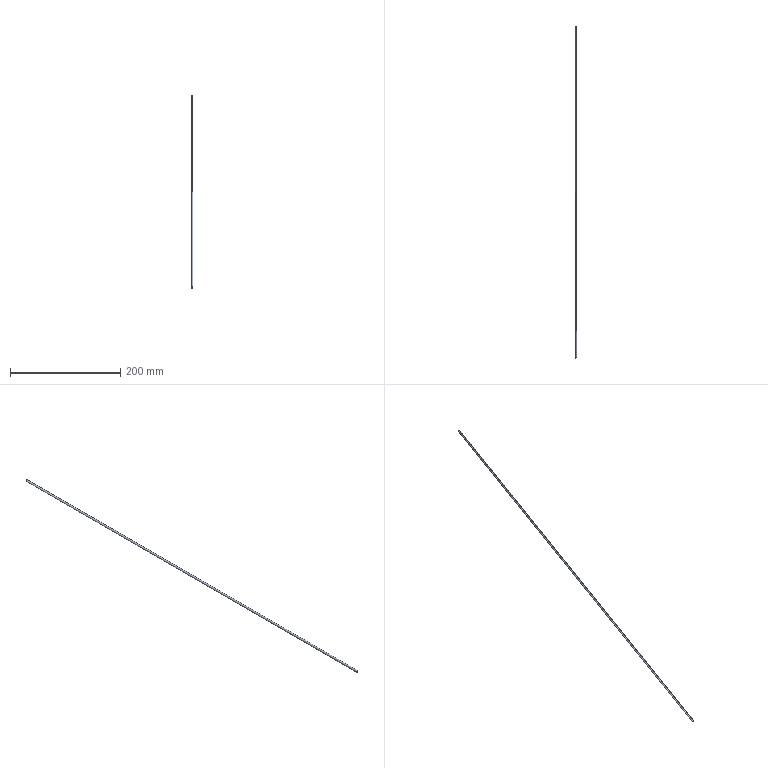Part | SolidWorks | features BaseBody 1 | 1 solid | 4 faces | box 3.2 x 601.041 x 348.507 mm | volume 5565 mm3 | cylinder 2 | plane 2 | commonest cylinder face diameters 3.2 x2
STEP:
#1=CARTESIAN_POINT('',(0.,659.718,2186.721));
#2=VERTEX_POINT('',#1);
#3=CARTESIAN_POINT('',(0.,661.317,2183.949));
#4=VERTEX_POINT('',#3);
#5=CARTESIAN_POINT('',(0.,660.518,2185.335));
#6=DIRECTION('',(0.,0.8662,0.4996));
#7=DIRECTION('',(0.,0.4996,-0.8662));
#8=AXIS2_PLACEMENT_3D('',#5,#6,#7);
#9=CIRCLE('',#8,1.6);
#10=EDGE_CURVE('',#2,#4,#9,.T.);
#11=ORIENTED_EDGE('',*,*,#10,.F.);
#12=CARTESIAN_POINT('',(0.,60.276,1840.985));
#13=VERTEX_POINT('',#12);
#14=CARTESIAN_POINT('',(0.,659.718,2186.721));
#15=DIRECTION('',(0.,-0.8662,-0.4996));
#16=VECTOR('',#15,1000.);
#17=LINE('',#14,#16);
#18=EDGE_CURVE('',#2,#13,#17,.T.);
#19=ORIENTED_EDGE('',*,*,#18,.T.);
#20=CARTESIAN_POINT('',(0.,61.875,1838.213));
#21=VERTEX_POINT('',#20);
#22=CARTESIAN_POINT('',(0.,61.075,1839.599));
#23=DIRECTION('',(0.,-0.8662,-0.4996));
#24=DIRECTION('',(0.,0.4996,-0.8662));
#25=AXIS2_PLACEMENT_3D('',#22,#23,#24);
#26=CIRCLE('',#25,1.6);
#27=EDGE_CURVE('',#21,#13,#26,.T.);
#28=ORIENTED_EDGE('',*,*,#27,.F.);
#29=CARTESIAN_POINT('',(0.,661.317,2183.949));
#30=DIRECTION('',(0.,-0.8662,-0.4996));
#31=VECTOR('',#30,1000.);
#32=LINE('',#29,#31);
#33=EDGE_CURVE('',#4,#21,#32,.T.);
#34=ORIENTED_EDGE('',*,*,#33,.F.);
#35=EDGE_LOOP('',(#11,#19,#28,#34));
#36=FACE_OUTER_BOUND('',#35,.T.);
#37=CARTESIAN_POINT('',(0.,660.518,2185.335));
#38=DIRECTION('',(0.,-0.8662,-0.4996));
#39=DIRECTION('',(0.,0.4996,-0.8662));
#40=AXIS2_PLACEMENT_3D('',#37,#38,#39);
#41=CYLINDRICAL_SURFACE('',#40,1.6);
#42=ADVANCED_FACE('',(#36),#41,.T.);
#43=ORIENTED_EDGE('',*,*,#18,.F.);
#44=CARTESIAN_POINT('',(0.,660.518,2185.335));
#45=DIRECTION('',(0.,0.8662,0.4996));
#46=DIRECTION('',(0.,0.4996,-0.8662));
#47=AXIS2_PLACEMENT_3D('',#44,#45,#46);
#48=CIRCLE('',#47,1.6);
#49=EDGE_CURVE('',#4,#2,#48,.T.);
#50=ORIENTED_EDGE('',*,*,#49,.F.);
#51=ORIENTED_EDGE('',*,*,#33,.T.);
#52=CARTESIAN_POINT('',(0.,61.075,1839.599));
#53=DIRECTION('',(0.,-0.8662,-0.4996));
#54=DIRECTION('',(0.,0.4996,-0.8662));
#55=AXIS2_PLACEMENT_3D('',#52,#53,#54);
#56=CIRCLE('',#55,1.6);
#57=EDGE_CURVE('',#13,#21,#56,.T.);
#58=ORIENTED_EDGE('',*,*,#57,.F.);
#59=EDGE_LOOP('',(#43,#50,#51,#58));
#60=FACE_OUTER_BOUND('',#59,.T.);
#61=CARTESIAN_POINT('',(0.,660.518,2185.335));
#62=DIRECTION('',(0.,-0.8662,-0.4996));
#63=DIRECTION('',(0.,0.4996,-0.8662));
#64=AXIS2_PLACEMENT_3D('',#61,#62,#63);
#65=CYLINDRICAL_SURFACE('',#64,1.6);
#66=ADVANCED_FACE('',(#60),#65,.T.);
#67=ORIENTED_EDGE('',*,*,#49,.T.);
#68=ORIENTED_EDGE('',*,*,#10,.T.);
#69=EDGE_LOOP('',(#67,#68));
#70=FACE_OUTER_BOUND('',#69,.T.);
#71=CARTESIAN_POINT('',(-1.619,661.327,2183.932));
#72=DIRECTION('',(0.,0.8662,0.4996));
#73=DIRECTION('',(0.,-0.4996,0.8662));
#74=AXIS2_PLACEMENT_3D('',#71,#72,#73);
#75=PLANE('',#74);
#76=ADVANCED_FACE('',(#70),#75,.T.);
#77=ORIENTED_EDGE('',*,*,#27,.T.);
#78=ORIENTED_EDGE('',*,*,#57,.T.);
#79=EDGE_LOOP('',(#77,#78));
#80=FACE_OUTER_BOUND('',#79,.T.);
#81=CARTESIAN_POINT('',(-1.619,61.884,1838.197));
#82=DIRECTION('',(0.,0.8662,0.4996));
#83=DIRECTION('',(0.,-0.4996,0.8662));
#84=AXIS2_PLACEMENT_3D('',#81,#82,#83);
#85=PLANE('',#84);
#86=ADVANCED_FACE('',(#80),#85,.F.);
#87=CLOSED_SHELL('',(#42,#66,#76,#86));
#88=MANIFOLD_SOLID_BREP('',#87);
#89=CARTESIAN_POINT('',(0.,0.,0.));
#90=DIRECTION('',(0.,0.,1.));
#91=DIRECTION('',(1.,0.,0.));
#92=AXIS2_PLACEMENT_3D('',#89,#90,#91);
#93=(LENGTH_UNIT()NAMED_UNIT(*)SI_UNIT(.MILLI.,.METRE.));
#94=UNCERTAINTY_MEASURE_WITH_UNIT(LENGTH_MEASURE(0.00001),#93,'','');
#95=(NAMED_UNIT(*)PLANE_ANGLE_UNIT()SI_UNIT($,.RADIAN.));
#96=(NAMED_UNIT(*)SI_UNIT($,.STERADIAN.)SOLID_ANGLE_UNIT());
#97=(GEOMETRIC_REPRESENTATION_CONTEXT(3)GLOBAL_UNCERTAINTY_ASSIGNED_CONTEXT((#94))GLOBAL_UNIT_ASSIGNED_CONTEXT((#93,#95,#96))REPRESENTATION_CONTEXT('',''));
#98=ADVANCED_BREP_SHAPE_REPRESENTATION('',(#88,#92),#97);